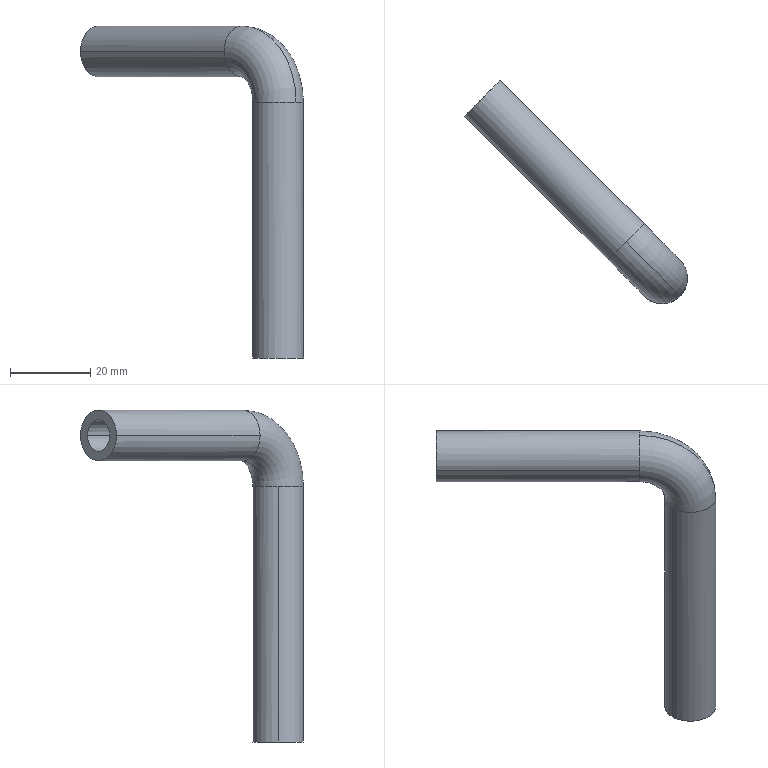Part | STEP file | Tube-500X095_1^Tube_6-P01_ASSEMBLY_KOMBAJN_OWOCOWY-003V11_Tube .500in OD X .095in Wall | 1 solid | 14 faces | box 55.673 x 55.673 x 82.885 mm | volume 10488 mm3 | cylinder 8 | torus 4 | plane 2 | commonest cylinder face diameters 7.874 x4 12.7 x4
STEP:
#1=CARTESIAN_POINT('',(0.,0.,0.));
#2=DIRECTION('',(0.,0.,1.));
#3=DIRECTION('',(1.,0.,0.));
#4=AXIS2_PLACEMENT_3D('',#1,#2,#3);
#5=CARTESIAN_POINT('',(3.937,0.,63.835));
#6=VERTEX_POINT('',#5);
#7=CARTESIAN_POINT('',(-2.784,2.784,63.835));
#8=VERTEX_POINT('',#7);
#9=CARTESIAN_POINT('',(0.,0.,63.835));
#10=DIRECTION('',(0.,0.,1.));
#11=DIRECTION('',(-1.,0.,0.));
#12=AXIS2_PLACEMENT_3D('',#9,#10,#11);
#13=CIRCLE('',#12,3.937);
#14=CARTESIAN_POINT('',(-8.98,8.98,63.835));
#15=DIRECTION('',(-0.7071,-0.7071,0.));
#16=DIRECTION('',(0.7071,-0.7071,0.));
#17=AXIS2_PLACEMENT_3D('',#14,#15,#16);
#18=TOROIDAL_SURFACE('',#17,12.7,3.937);
#19=CARTESIAN_POINT('',(0.,8.639));
#20=DIRECTION('',(0.,-1.));
#21=VECTOR('',#20,1.);
#22=LINE('',#19,#21);
#23=(GEOMETRIC_REPRESENTATION_CONTEXT(2)PARAMETRIC_REPRESENTATION_CONTEXT()REPRESENTATION_CONTEXT('',''));
#24=DEFINITIONAL_REPRESENTATION('',(#22),#23);
#25=PCURVE('',#18,#24);
#26=CARTESIAN_POINT('',(0.,0.,63.835));
#27=DIRECTION('',(0.,0.,-1.));
#28=DIRECTION('',(-1.,0.,0.));
#29=AXIS2_PLACEMENT_3D('',#26,#27,#28);
#30=CYLINDRICAL_SURFACE('',#29,3.937);
#31=CARTESIAN_POINT('',(6.283,0.));
#32=DIRECTION('',(-1.,0.));
#33=VECTOR('',#32,1.);
#34=LINE('',#31,#33);
#35=(GEOMETRIC_REPRESENTATION_CONTEXT(2)PARAMETRIC_REPRESENTATION_CONTEXT()REPRESENTATION_CONTEXT('',''));
#36=DEFINITIONAL_REPRESENTATION('',(#34),#35);
#37=PCURVE('',#30,#36);
#38=SURFACE_CURVE('',#13,(#25,#37),.PCURVE_S1.);
#39=EDGE_CURVE('',#6,#8,#38,.T.);
#40=ORIENTED_EDGE('',*,*,#39,.T.);
#41=CARTESIAN_POINT('',(-8.98,8.98,72.598));
#42=VERTEX_POINT('',#41);
#43=CARTESIAN_POINT('',(-8.98,8.98,63.835));
#44=DIRECTION('',(-0.7071,-0.7071,0.));
#45=DIRECTION('',(0.7071,-0.7071,0.));
#46=AXIS2_PLACEMENT_3D('',#43,#44,#45);
#47=CIRCLE('',#46,8.763);
#48=CARTESIAN_POINT('',(0.,3.142));
#49=DIRECTION('',(1.,0.));
#50=VECTOR('',#49,1.);
#51=LINE('',#48,#50);
#52=(GEOMETRIC_REPRESENTATION_CONTEXT(2)PARAMETRIC_REPRESENTATION_CONTEXT()REPRESENTATION_CONTEXT('',''));
#53=DEFINITIONAL_REPRESENTATION('',(#51),#52);
#54=PCURVE('',#18,#53);
#55=CARTESIAN_POINT('',(-8.98,8.98,63.835));
#56=DIRECTION('',(-0.7071,-0.7071,0.));
#57=DIRECTION('',(0.7071,-0.7071,0.));
#58=AXIS2_PLACEMENT_3D('',#55,#56,#57);
#59=TOROIDAL_SURFACE('',#58,12.7,3.937);
#60=CARTESIAN_POINT('',(0.,3.142));
#61=DIRECTION('',(1.,0.));
#62=VECTOR('',#61,1.);
#63=LINE('',#60,#62);
#64=(GEOMETRIC_REPRESENTATION_CONTEXT(2)PARAMETRIC_REPRESENTATION_CONTEXT()REPRESENTATION_CONTEXT('',''));
#65=DEFINITIONAL_REPRESENTATION('',(#63),#64);
#66=PCURVE('',#59,#65);
#67=SURFACE_CURVE('',#47,(#54,#66),.PCURVE_S1.);
#68=EDGE_CURVE('',#8,#42,#67,.T.);
#69=ORIENTED_EDGE('',*,*,#68,.T.);
#70=CARTESIAN_POINT('',(-6.196,11.764,76.535));
#71=VERTEX_POINT('',#70);
#72=CARTESIAN_POINT('',(-8.98,8.98,76.535));
#73=DIRECTION('',(-0.7071,0.7071,0.));
#74=DIRECTION('',(-0.7071,-0.7071,0.));
#75=AXIS2_PLACEMENT_3D('',#72,#73,#74);
#76=CIRCLE('',#75,3.937);
#77=CARTESIAN_POINT('',(1.571,7.854));
#78=DIRECTION('',(0.,-1.));
#79=VECTOR('',#78,1.);
#80=LINE('',#77,#79);
#81=(GEOMETRIC_REPRESENTATION_CONTEXT(2)PARAMETRIC_REPRESENTATION_CONTEXT()REPRESENTATION_CONTEXT('',''));
#82=DEFINITIONAL_REPRESENTATION('',(#80),#81);
#83=PCURVE('',#18,#82);
#84=CARTESIAN_POINT('',(-8.98,8.98,76.535));
#85=DIRECTION('',(-0.7071,0.7071,0.));
#86=DIRECTION('',(-0.7071,-0.7071,0.));
#87=AXIS2_PLACEMENT_3D('',#84,#85,#86);
#88=CYLINDRICAL_SURFACE('',#87,3.937);
#89=CARTESIAN_POINT('',(0.,0.));
#90=DIRECTION('',(1.,0.));
#91=VECTOR('',#90,1.);
#92=LINE('',#89,#91);
#93=(GEOMETRIC_REPRESENTATION_CONTEXT(2)PARAMETRIC_REPRESENTATION_CONTEXT()REPRESENTATION_CONTEXT('',''));
#94=DEFINITIONAL_REPRESENTATION('',(#92),#93);
#95=PCURVE('',#88,#94);
#96=SURFACE_CURVE('',#76,(#83,#95),.PCURVE_S1.);
#97=EDGE_CURVE('',#71,#42,#96,.T.);
#98=ORIENTED_EDGE('',*,*,#97,.F.);
#99=CARTESIAN_POINT('',(-8.98,8.98,80.472));
#100=VERTEX_POINT('',#99);
#101=CARTESIAN_POINT('',(-8.98,8.98,76.535));
#102=DIRECTION('',(-0.7071,0.7071,0.));
#103=DIRECTION('',(-0.7071,-0.7071,0.));
#104=AXIS2_PLACEMENT_3D('',#101,#102,#103);
#105=CIRCLE('',#104,3.937);
#106=CARTESIAN_POINT('',(1.571,7.854));
#107=DIRECTION('',(0.,-1.));
#108=VECTOR('',#107,1.);
#109=LINE('',#106,#108);
#110=(GEOMETRIC_REPRESENTATION_CONTEXT(2)PARAMETRIC_REPRESENTATION_CONTEXT()REPRESENTATION_CONTEXT('',''));
#111=DEFINITIONAL_REPRESENTATION('',(#109),#110);
#112=PCURVE('',#18,#111);
#113=CARTESIAN_POINT('',(-8.98,8.98,76.535));
#114=DIRECTION('',(-0.7071,0.7071,0.));
#115=DIRECTION('',(-0.7071,-0.7071,0.));
#116=AXIS2_PLACEMENT_3D('',#113,#114,#115);
#117=CYLINDRICAL_SURFACE('',#116,3.937);
#118=CARTESIAN_POINT('',(0.,0.));
#119=DIRECTION('',(1.,0.));
#120=VECTOR('',#119,1.);
#121=LINE('',#118,#120);
#122=(GEOMETRIC_REPRESENTATION_CONTEXT(2)PARAMETRIC_REPRESENTATION_CONTEXT()REPRESENTATION_CONTEXT('',''));
#123=DEFINITIONAL_REPRESENTATION('',(#121),#122);
#124=PCURVE('',#117,#123);
#125=SURFACE_CURVE('',#105,(#112,#124),.PCURVE_S1.);
#126=EDGE_CURVE('',#100,#71,#125,.T.);
#127=ORIENTED_EDGE('',*,*,#126,.F.);
#128=CARTESIAN_POINT('',(2.784,-2.784,63.835));
#129=VERTEX_POINT('',#128);
#130=CARTESIAN_POINT('',(-8.98,8.98,63.835));
#131=DIRECTION('',(-0.7071,-0.7071,0.));
#132=DIRECTION('',(0.7071,-0.7071,0.));
#133=AXIS2_PLACEMENT_3D('',#130,#131,#132);
#134=CIRCLE('',#133,16.637);
#135=CARTESIAN_POINT('',(0.,6.283));
#136=DIRECTION('',(1.,0.));
#137=VECTOR('',#136,1.);
#138=LINE('',#135,#137);
#139=(GEOMETRIC_REPRESENTATION_CONTEXT(2)PARAMETRIC_REPRESENTATION_CONTEXT()REPRESENTATION_CONTEXT('',''));
#140=DEFINITIONAL_REPRESENTATION('',(#138),#139);
#141=PCURVE('',#18,#140);
#142=CARTESIAN_POINT('',(0.,0.));
#143=DIRECTION('',(1.,0.));
#144=VECTOR('',#143,1.);
#145=LINE('',#142,#144);
#146=(GEOMETRIC_REPRESENTATION_CONTEXT(2)PARAMETRIC_REPRESENTATION_CONTEXT()REPRESENTATION_CONTEXT('',''));
#147=DEFINITIONAL_REPRESENTATION('',(#145),#146);
#148=PCURVE('',#59,#147);
#149=SURFACE_CURVE('',#134,(#141,#148),.PCURVE_S1.);
#150=EDGE_CURVE('',#129,#100,#149,.T.);
#151=ORIENTED_EDGE('',*,*,#150,.F.);
#152=CARTESIAN_POINT('',(0.,0.,63.835));
#153=DIRECTION('',(0.,0.,1.));
#154=DIRECTION('',(-1.,0.,0.));
#155=AXIS2_PLACEMENT_3D('',#152,#153,#154);
#156=CIRCLE('',#155,3.937);
#157=CARTESIAN_POINT('',(0.,8.639));
#158=DIRECTION('',(0.,-1.));
#159=VECTOR('',#158,1.);
#160=LINE('',#157,#159);
#161=(GEOMETRIC_REPRESENTATION_CONTEXT(2)PARAMETRIC_REPRESENTATION_CONTEXT()REPRESENTATION_CONTEXT('',''));
#162=DEFINITIONAL_REPRESENTATION('',(#160),#161);
#163=PCURVE('',#18,#162);
#164=CARTESIAN_POINT('',(0.,0.,63.835));
#165=DIRECTION('',(0.,0.,-1.));
#166=DIRECTION('',(-1.,0.,0.));
#167=AXIS2_PLACEMENT_3D('',#164,#165,#166);
#168=CYLINDRICAL_SURFACE('',#167,3.937);
#169=CARTESIAN_POINT('',(6.283,0.));
#170=DIRECTION('',(-1.,0.));
#171=VECTOR('',#170,1.);
#172=LINE('',#169,#171);
#173=(GEOMETRIC_REPRESENTATION_CONTEXT(2)PARAMETRIC_REPRESENTATION_CONTEXT()REPRESENTATION_CONTEXT('',''));
#174=DEFINITIONAL_REPRESENTATION('',(#172),#173);
#175=PCURVE('',#168,#174);
#176=SURFACE_CURVE('',#156,(#163,#175),.PCURVE_S1.);
#177=EDGE_CURVE('',#129,#6,#176,.T.);
#178=ORIENTED_EDGE('',*,*,#177,.T.);
#179=EDGE_LOOP('',(#40,#69,#98,#127,#151,#178));
#180=FACE_BOUND('',#179,.F.);
#181=ADVANCED_FACE('',(#180),#18,.F.);
#182=CARTESIAN_POINT('',(-6.35,0.,63.835));
#183=VERTEX_POINT('',#182);
#184=CARTESIAN_POINT('',(4.49,-4.49,63.835));
#185=VERTEX_POINT('',#184);
#186=CARTESIAN_POINT('',(0.,0.,63.835));
#187=DIRECTION('',(0.,0.,1.));
#188=DIRECTION('',(1.,0.,0.));
#189=AXIS2_PLACEMENT_3D('',#186,#187,#188);
#190=CIRCLE('',#189,6.35);
#191=CARTESIAN_POINT('',(-8.98,8.98,63.835));
#192=DIRECTION('',(-0.7071,-0.7071,0.));
#193=DIRECTION('',(0.7071,-0.7071,0.));
#194=AXIS2_PLACEMENT_3D('',#191,#192,#193);
#195=TOROIDAL_SURFACE('',#194,12.7,6.35);
#196=CARTESIAN_POINT('',(0.,5.498));
#197=DIRECTION('',(0.,-1.));
#198=VECTOR('',#197,1.);
#199=LINE('',#196,#198);
#200=(GEOMETRIC_REPRESENTATION_CONTEXT(2)PARAMETRIC_REPRESENTATION_CONTEXT()REPRESENTATION_CONTEXT('',''));
#201=DEFINITIONAL_REPRESENTATION('',(#199),#200);
#202=PCURVE('',#195,#201);
#203=CARTESIAN_POINT('',(0.,0.,63.835));
#204=DIRECTION('',(0.,0.,-1.));
#205=DIRECTION('',(-1.,0.,0.));
#206=AXIS2_PLACEMENT_3D('',#203,#204,#205);
#207=CYLINDRICAL_SURFACE('',#206,6.35);
#208=CARTESIAN_POINT('',(9.425,0.));
#209=DIRECTION('',(-1.,0.));
#210=VECTOR('',#209,1.);
#211=LINE('',#208,#210);
#212=(GEOMETRIC_REPRESENTATION_CONTEXT(2)PARAMETRIC_REPRESENTATION_CONTEXT()REPRESENTATION_CONTEXT('',''));
#213=DEFINITIONAL_REPRESENTATION('',(#211),#212);
#214=PCURVE('',#207,#213);
#215=SURFACE_CURVE('',#190,(#202,#214),.PCURVE_S1.);
#216=EDGE_CURVE('',#183,#185,#215,.T.);
#217=ORIENTED_EDGE('',*,*,#216,.T.);
#218=CARTESIAN_POINT('',(-8.98,8.98,82.885));
#219=VERTEX_POINT('',#218);
#220=CARTESIAN_POINT('',(-8.98,8.98,63.835));
#221=DIRECTION('',(-0.7071,-0.7071,0.));
#222=DIRECTION('',(0.7071,-0.7071,0.));
#223=AXIS2_PLACEMENT_3D('',#220,#221,#222);
#224=CIRCLE('',#223,19.05);
#225=CARTESIAN_POINT('',(0.,0.));
#226=DIRECTION('',(1.,0.));
#227=VECTOR('',#226,1.);
#228=LINE('',#225,#227);
#229=(GEOMETRIC_REPRESENTATION_CONTEXT(2)PARAMETRIC_REPRESENTATION_CONTEXT()REPRESENTATION_CONTEXT('',''));
#230=DEFINITIONAL_REPRESENTATION('',(#228),#229);
#231=PCURVE('',#195,#230);
#232=CARTESIAN_POINT('',(-8.98,8.98,63.835));
#233=DIRECTION('',(-0.7071,-0.7071,0.));
#234=DIRECTION('',(0.7071,-0.7071,0.));
#235=AXIS2_PLACEMENT_3D('',#232,#233,#234);
#236=TOROIDAL_SURFACE('',#235,12.7,6.35);
#237=CARTESIAN_POINT('',(0.,6.283));
#238=CARTESIAN_POINT('',(0.0238,6.283));
#239=CARTESIAN_POINT('',(0.0714,6.283));
#240=CARTESIAN_POINT('',(0.1428,6.283));
#241=CARTESIAN_POINT('',(0.2142,6.283));
#242=CARTESIAN_POINT('',(0.2856,6.283));
#243=CARTESIAN_POINT('',(0.357,6.283));
#244=CARTESIAN_POINT('',(0.4284,6.283));
#245=CARTESIAN_POINT('',(0.4998,6.283));
#246=CARTESIAN_POINT('',(0.5712,6.283));
#247=CARTESIAN_POINT('',(0.6426,6.283));
#248=CARTESIAN_POINT('',(0.714,6.283));
#249=CARTESIAN_POINT('',(0.7854,6.283));
#250=CARTESIAN_POINT('',(0.8568,6.283));
#251=CARTESIAN_POINT('',(0.9282,6.283));
#252=CARTESIAN_POINT('',(0.9996,6.283));
#253=CARTESIAN_POINT('',(1.071,6.283));
#254=CARTESIAN_POINT('',(1.142,6.283));
#255=CARTESIAN_POINT('',(1.214,6.283));
#256=CARTESIAN_POINT('',(1.285,6.283));
#257=CARTESIAN_POINT('',(1.357,6.283));
#258=CARTESIAN_POINT('',(1.428,6.283));
#259=CARTESIAN_POINT('',(1.499,6.283));
#260=CARTESIAN_POINT('',(1.547,6.283));
#261=CARTESIAN_POINT('',(1.571,6.283));
#262=B_SPLINE_CURVE_WITH_KNOTS('',3,(#237,#238,#239,#240,#241,#242,#243,#244,#245,#246,#247,#248,#249,#250,#251,#252,#253,#254,#255,#256,#257,#258,#259,#260,#261),.UNSPECIFIED.,.F.,.F.,(4,1,1,1,1,1,1,1,1,1,1,1,1,1,1,1,1,1,1,1,1,1,4),(0.,0.0714,0.1428,0.2142,0.2856,0.357,0.4284,0.4998,0.5712,0.6426,0.714,0.7854,0.8568,0.9282,0.9996,1.071,1.142,1.214,1.285,1.357,1.428,1.499,1.571),.QUASI_UNIFORM_KNOTS.);
#263=(GEOMETRIC_REPRESENTATION_CONTEXT(2)PARAMETRIC_REPRESENTATION_CONTEXT()REPRESENTATION_CONTEXT('',''));
#264=DEFINITIONAL_REPRESENTATION('',(#262),#263);
#265=PCURVE('',#236,#264);
#266=SURFACE_CURVE('',#224,(#231,#265),.PCURVE_S1.);
#267=EDGE_CURVE('',#185,#219,#266,.T.);
#268=ORIENTED_EDGE('',*,*,#267,.T.);
#269=CARTESIAN_POINT('',(-13.47,4.49,76.535));
#270=VERTEX_POINT('',#269);
#271=CARTESIAN_POINT('',(-8.98,8.98,76.535));
#272=DIRECTION('',(-0.7071,0.7071,0.));
#273=DIRECTION('',(0.5,0.5,0.7071));
#274=AXIS2_PLACEMENT_3D('',#271,#272,#273);
#275=CIRCLE('',#274,6.35);
#276=CARTESIAN_POINT('',(1.571,5.498));
#277=DIRECTION('',(0.,-1.));
#278=VECTOR('',#277,1.);
#279=LINE('',#276,#278);
#280=(GEOMETRIC_REPRESENTATION_CONTEXT(2)PARAMETRIC_REPRESENTATION_CONTEXT()REPRESENTATION_CONTEXT('',''));
#281=DEFINITIONAL_REPRESENTATION('',(#279),#280);
#282=PCURVE('',#195,#281);
#283=CARTESIAN_POINT('',(-8.98,8.98,76.535));
#284=DIRECTION('',(-0.7071,0.7071,0.));
#285=DIRECTION('',(-0.7071,-0.7071,0.));
#286=AXIS2_PLACEMENT_3D('',#283,#284,#285);
#287=CYLINDRICAL_SURFACE('',#286,6.35);
#288=CARTESIAN_POINT('',(-3.927,0.));
#289=DIRECTION('',(1.,0.));
#290=VECTOR('',#289,1.);
#291=LINE('',#288,#290);
#292=(GEOMETRIC_REPRESENTATION_CONTEXT(2)PARAMETRIC_REPRESENTATION_CONTEXT()REPRESENTATION_CONTEXT('',''));
#293=DEFINITIONAL_REPRESENTATION('',(#291),#292);
#294=PCURVE('',#287,#293);
#295=SURFACE_CURVE('',#275,(#282,#294),.PCURVE_S1.);
#296=EDGE_CURVE('',#270,#219,#295,.T.);
#297=ORIENTED_EDGE('',*,*,#296,.F.);
#298=CARTESIAN_POINT('',(-8.98,8.98,70.185));
#299=VERTEX_POINT('',#298);
#300=CARTESIAN_POINT('',(-8.98,8.98,76.535));
#301=DIRECTION('',(-0.7071,0.7071,0.));
#302=DIRECTION('',(0.5,0.5,0.7071));
#303=AXIS2_PLACEMENT_3D('',#300,#301,#302);
#304=CIRCLE('',#303,6.35);
#305=CARTESIAN_POINT('',(1.571,5.498));
#306=DIRECTION('',(0.,-1.));
#307=VECTOR('',#306,1.);
#308=LINE('',#305,#307);
#309=(GEOMETRIC_REPRESENTATION_CONTEXT(2)PARAMETRIC_REPRESENTATION_CONTEXT()REPRESENTATION_CONTEXT('',''));
#310=DEFINITIONAL_REPRESENTATION('',(#308),#309);
#311=PCURVE('',#195,#310);
#312=CARTESIAN_POINT('',(-8.98,8.98,76.535));
#313=DIRECTION('',(-0.7071,0.7071,0.));
#314=DIRECTION('',(-0.7071,-0.7071,0.));
#315=AXIS2_PLACEMENT_3D('',#312,#313,#314);
#316=CYLINDRICAL_SURFACE('',#315,6.35);
#317=CARTESIAN_POINT('',(2.356,0.));
#318=DIRECTION('',(1.,0.));
#319=VECTOR('',#318,1.);
#320=LINE('',#317,#319);
#321=(GEOMETRIC_REPRESENTATION_CONTEXT(2)PARAMETRIC_REPRESENTATION_CONTEXT()REPRESENTATION_CONTEXT('',''));
#322=DEFINITIONAL_REPRESENTATION('',(#320),#321);
#323=PCURVE('',#316,#322);
#324=SURFACE_CURVE('',#304,(#311,#323),.PCURVE_S1.);
#325=EDGE_CURVE('',#299,#270,#324,.T.);
#326=ORIENTED_EDGE('',*,*,#325,.F.);
#327=CARTESIAN_POINT('',(-4.49,4.49,63.835));
#328=VERTEX_POINT('',#327);
#329=CARTESIAN_POINT('',(-8.98,8.98,63.835));
#330=DIRECTION('',(-0.7071,-0.7071,0.));
#331=DIRECTION('',(0.7071,-0.7071,0.));
#332=AXIS2_PLACEMENT_3D('',#329,#330,#331);
#333=CIRCLE('',#332,6.35);
#334=CARTESIAN_POINT('',(0.,3.142));
#335=DIRECTION('',(1.,0.));
#336=VECTOR('',#335,1.);
#337=LINE('',#334,#336);
#338=(GEOMETRIC_REPRESENTATION_CONTEXT(2)PARAMETRIC_REPRESENTATION_CONTEXT()REPRESENTATION_CONTEXT('',''));
#339=DEFINITIONAL_REPRESENTATION('',(#337),#338);
#340=PCURVE('',#195,#339);
#341=CARTESIAN_POINT('',(0.,3.142));
#342=DIRECTION('',(1.,0.));
#343=VECTOR('',#342,1.);
#344=LINE('',#341,#343);
#345=(GEOMETRIC_REPRESENTATION_CONTEXT(2)PARAMETRIC_REPRESENTATION_CONTEXT()REPRESENTATION_CONTEXT('',''));
#346=DEFINITIONAL_REPRESENTATION('',(#344),#345);
#347=PCURVE('',#236,#346);
#348=SURFACE_CURVE('',#333,(#340,#347),.PCURVE_S1.);
#349=EDGE_CURVE('',#328,#299,#348,.T.);
#350=ORIENTED_EDGE('',*,*,#349,.F.);
#351=CARTESIAN_POINT('',(0.,0.,63.835));
#352=DIRECTION('',(0.,0.,1.));
#353=DIRECTION('',(1.,0.,0.));
#354=AXIS2_PLACEMENT_3D('',#351,#352,#353);
#355=CIRCLE('',#354,6.35);
#356=CARTESIAN_POINT('',(0.,5.498));
#357=DIRECTION('',(0.,-1.));
#358=VECTOR('',#357,1.);
#359=LINE('',#356,#358);
#360=(GEOMETRIC_REPRESENTATION_CONTEXT(2)PARAMETRIC_REPRESENTATION_CONTEXT()REPRESENTATION_CONTEXT('',''));
#361=DEFINITIONAL_REPRESENTATION('',(#359),#360);
#362=PCURVE('',#195,#361);
#363=CARTESIAN_POINT('',(0.,0.,63.835));
#364=DIRECTION('',(0.,0.,-1.));
#365=DIRECTION('',(-1.,0.,0.));
#366=AXIS2_PLACEMENT_3D('',#363,#364,#365);
#367=CYLINDRICAL_SURFACE('',#366,6.35);
#368=CARTESIAN_POINT('',(3.142,0.));
#369=DIRECTION('',(-1.,0.));
#370=VECTOR('',#369,1.);
#371=LINE('',#368,#370);
#372=(GEOMETRIC_REPRESENTATION_CONTEXT(2)PARAMETRIC_REPRESENTATION_CONTEXT()REPRESENTATION_CONTEXT('',''));
#373=DEFINITIONAL_REPRESENTATION('',(#371),#372);
#374=PCURVE('',#367,#373);
#375=SURFACE_CURVE('',#355,(#362,#374),.PCURVE_S1.);
#376=EDGE_CURVE('',#328,#183,#375,.T.);
#377=ORIENTED_EDGE('',*,*,#376,.T.);
#378=EDGE_LOOP('',(#217,#268,#297,#326,#350,#377));
#379=FACE_BOUND('',#378,.T.);
#380=ADVANCED_FACE('',(#379),#195,.T.);
#381=CARTESIAN_POINT('',(-3.937,0.,63.835));
#382=VERTEX_POINT('',#381);
#383=CARTESIAN_POINT('',(-3.937,0.,0.));
#384=VERTEX_POINT('',#383);
#385=CARTESIAN_POINT('',(-3.937,0.,63.835));
#386=DIRECTION('',(0.,0.,-1.));
#387=VECTOR('',#386,1.);
#388=LINE('',#385,#387);
#389=CARTESIAN_POINT('',(6.283,0.));
#390=DIRECTION('',(0.,1.));
#391=VECTOR('',#390,1.);
#392=LINE('',#389,#391);
#393=(GEOMETRIC_REPRESENTATION_CONTEXT(2)PARAMETRIC_REPRESENTATION_CONTEXT()REPRESENTATION_CONTEXT('',''));
#394=DEFINITIONAL_REPRESENTATION('',(#392),#393);
#395=PCURVE('',#168,#394);
#396=CARTESIAN_POINT('',(0.,0.));
#397=DIRECTION('',(0.,1.));
#398=VECTOR('',#397,1.);
#399=LINE('',#396,#398);
#400=(GEOMETRIC_REPRESENTATION_CONTEXT(2)PARAMETRIC_REPRESENTATION_CONTEXT()REPRESENTATION_CONTEXT('',''));
#401=DEFINITIONAL_REPRESENTATION('',(#399),#400);
#402=PCURVE('',#30,#401);
#403=SURFACE_CURVE('',#388,(#395,#402),.PCURVE_S1.);
#404=EDGE_CURVE('',#382,#384,#403,.T.);
#405=ORIENTED_EDGE('',*,*,#404,.T.);
#406=CARTESIAN_POINT('',(3.937,0.,0.));
#407=VERTEX_POINT('',#406);
#408=CARTESIAN_POINT('',(0.,0.,0.));
#409=DIRECTION('',(0.,0.,1.));
#410=DIRECTION('',(1.,0.,0.));
#411=AXIS2_PLACEMENT_3D('',#408,#409,#410);
#412=CIRCLE('',#411,3.937);
#413=CARTESIAN_POINT('',(9.425,63.835));
#414=DIRECTION('',(-1.,0.));
#415=VECTOR('',#414,1.);
#416=LINE('',#413,#415);
#417=(GEOMETRIC_REPRESENTATION_CONTEXT(2)PARAMETRIC_REPRESENTATION_CONTEXT()REPRESENTATION_CONTEXT('',''));
#418=DEFINITIONAL_REPRESENTATION('',(#416),#417);
#419=PCURVE('',#168,#418);
#420=CARTESIAN_POINT('',(0.,0.,0.));
#421=DIRECTION('',(0.,0.,1.));
#422=DIRECTION('',(1.,0.,0.));
#423=AXIS2_PLACEMENT_3D('',#420,#421,#422);
#424=PLANE('',#423);
#425=CARTESIAN_POINT('',(0.,0.));
#426=DIRECTION('',(1.,0.));
#427=AXIS2_PLACEMENT_2D('',#425,#426);
#428=CIRCLE('',#427,3.937);
#429=(GEOMETRIC_REPRESENTATION_CONTEXT(2)PARAMETRIC_REPRESENTATION_CONTEXT()REPRESENTATION_CONTEXT('',''));
#430=DEFINITIONAL_REPRESENTATION('',(#428),#429);
#431=PCURVE('',#424,#430);
#432=SURFACE_CURVE('',#412,(#419,#431),.PCURVE_S1.);
#433=EDGE_CURVE('',#384,#407,#432,.T.);
#434=ORIENTED_EDGE('',*,*,#433,.T.);
#435=CARTESIAN_POINT('',(3.937,0.,63.835));
#436=DIRECTION('',(0.,0.,-1.));
#437=VECTOR('',#436,1.);
#438=LINE('',#435,#437);
#439=CARTESIAN_POINT('',(3.142,0.));
#440=DIRECTION('',(0.,1.));
#441=VECTOR('',#440,1.);
#442=LINE('',#439,#441);
#443=(GEOMETRIC_REPRESENTATION_CONTEXT(2)PARAMETRIC_REPRESENTATION_CONTEXT()REPRESENTATION_CONTEXT('',''));
#444=DEFINITIONAL_REPRESENTATION('',(#442),#443);
#445=PCURVE('',#168,#444);
#446=CARTESIAN_POINT('',(3.142,0.));
#447=DIRECTION('',(0.,1.));
#448=VECTOR('',#447,1.);
#449=LINE('',#446,#448);
#450=(GEOMETRIC_REPRESENTATION_CONTEXT(2)PARAMETRIC_REPRESENTATION_CONTEXT()REPRESENTATION_CONTEXT('',''));
#451=DEFINITIONAL_REPRESENTATION('',(#449),#450);
#452=PCURVE('',#30,#451);
#453=SURFACE_CURVE('',#438,(#445,#452),.PCURVE_S1.);
#454=EDGE_CURVE('',#6,#407,#453,.T.);
#455=ORIENTED_EDGE('',*,*,#454,.F.);
#456=ORIENTED_EDGE('',*,*,#177,.F.);
#457=CARTESIAN_POINT('',(0.,0.,63.835));
#458=DIRECTION('',(0.,0.,1.));
#459=DIRECTION('',(-1.,0.,0.));
#460=AXIS2_PLACEMENT_3D('',#457,#458,#459);
#461=CIRCLE('',#460,3.937);
#462=CARTESIAN_POINT('',(6.283,0.));
#463=DIRECTION('',(-1.,0.));
#464=VECTOR('',#463,1.);
#465=LINE('',#462,#464);
#466=(GEOMETRIC_REPRESENTATION_CONTEXT(2)PARAMETRIC_REPRESENTATION_CONTEXT()REPRESENTATION_CONTEXT('',''));
#467=DEFINITIONAL_REPRESENTATION('',(#465),#466);
#468=PCURVE('',#168,#467);
#469=CARTESIAN_POINT('',(0.,2.356));
#470=DIRECTION('',(0.,-1.));
#471=VECTOR('',#470,1.);
#472=LINE('',#469,#471);
#473=(GEOMETRIC_REPRESENTATION_CONTEXT(2)PARAMETRIC_REPRESENTATION_CONTEXT()REPRESENTATION_CONTEXT('',''));
#474=DEFINITIONAL_REPRESENTATION('',(#472),#473);
#475=PCURVE('',#59,#474);
#476=SURFACE_CURVE('',#461,(#468,#475),.PCURVE_S1.);
#477=EDGE_CURVE('',#382,#129,#476,.T.);
#478=ORIENTED_EDGE('',*,*,#477,.F.);
#479=EDGE_LOOP('',(#405,#434,#455,#456,#478));
#480=FACE_BOUND('',#479,.F.);
#481=ADVANCED_FACE('',(#480),#168,.F.);
#482=CARTESIAN_POINT('',(-11.764,6.196,76.535));
#483=VERTEX_POINT('',#482);
#484=CARTESIAN_POINT('',(-8.98,8.98,76.535));
#485=DIRECTION('',(-0.7071,0.7071,0.));
#486=DIRECTION('',(-0.7071,-0.7071,0.));
#487=AXIS2_PLACEMENT_3D('',#484,#485,#486);
#488=CIRCLE('',#487,3.937);
#489=CARTESIAN_POINT('',(0.,0.));
#490=DIRECTION('',(1.,0.));
#491=VECTOR('',#490,1.);
#492=LINE('',#489,#491);
#493=(GEOMETRIC_REPRESENTATION_CONTEXT(2)PARAMETRIC_REPRESENTATION_CONTEXT()REPRESENTATION_CONTEXT('',''));
#494=DEFINITIONAL_REPRESENTATION('',(#492),#493);
#495=PCURVE('',#88,#494);
#496=CARTESIAN_POINT('',(1.571,7.854));
#497=DIRECTION('',(0.,-1.));
#498=VECTOR('',#497,1.);
#499=LINE('',#496,#498);
#500=(GEOMETRIC_REPRESENTATION_CONTEXT(2)PARAMETRIC_REPRESENTATION_CONTEXT()REPRESENTATION_CONTEXT('',''));
#501=DEFINITIONAL_REPRESENTATION('',(#499),#500);
#502=PCURVE('',#59,#501);
#503=SURFACE_CURVE('',#488,(#495,#502),.PCURVE_S1.);
#504=EDGE_CURVE('',#42,#483,#503,.T.);
#505=ORIENTED_EDGE('',*,*,#504,.T.);
#506=CARTESIAN_POINT('',(-47.616,42.049,76.535));
#507=VERTEX_POINT('',#506);
#508=CARTESIAN_POINT('',(-11.764,6.196,76.535));
#509=DIRECTION('',(-0.7071,0.7071,0.));
#510=VECTOR('',#509,1.);
#511=LINE('',#508,#510);
#512=CARTESIAN_POINT('',(6.283,0.));
#513=DIRECTION('',(0.,1.));
#514=VECTOR('',#513,1.);
#515=LINE('',#512,#514);
#516=(GEOMETRIC_REPRESENTATION_CONTEXT(2)PARAMETRIC_REPRESENTATION_CONTEXT()REPRESENTATION_CONTEXT('',''));
#517=DEFINITIONAL_REPRESENTATION('',(#515),#516);
#518=PCURVE('',#88,#517);
#519=CARTESIAN_POINT('',(0.,0.));
#520=DIRECTION('',(0.,1.));
#521=VECTOR('',#520,1.);
#522=LINE('',#519,#521);
#523=(GEOMETRIC_REPRESENTATION_CONTEXT(2)PARAMETRIC_REPRESENTATION_CONTEXT()REPRESENTATION_CONTEXT('',''));
#524=DEFINITIONAL_REPRESENTATION('',(#522),#523);
#525=PCURVE('',#117,#524);
#526=SURFACE_CURVE('',#511,(#518,#525),.PCURVE_S1.);
#527=EDGE_CURVE('',#483,#507,#526,.T.);
#528=ORIENTED_EDGE('',*,*,#527,.T.);
#529=CARTESIAN_POINT('',(-42.049,47.616,76.535));
#530=VERTEX_POINT('',#529);
#531=CARTESIAN_POINT('',(-44.832,44.832,76.535));
#532=DIRECTION('',(-0.7071,0.7071,0.));
#533=DIRECTION('',(-0.7071,-0.7071,0.));
#534=AXIS2_PLACEMENT_3D('',#531,#532,#533);
#535=CIRCLE('',#534,3.937);
#536=CARTESIAN_POINT('',(0.,50.703));
#537=DIRECTION('',(1.,0.));
#538=VECTOR('',#537,1.);
#539=LINE('',#536,#538);
#540=(GEOMETRIC_REPRESENTATION_CONTEXT(2)PARAMETRIC_REPRESENTATION_CONTEXT()REPRESENTATION_CONTEXT('',''));
#541=DEFINITIONAL_REPRESENTATION('',(#539),#540);
#542=PCURVE('',#88,#541);
#543=CARTESIAN_POINT('',(-44.832,44.832,76.535));
#544=DIRECTION('',(-0.7071,0.7071,0.));
#545=DIRECTION('',(0.5,0.5,0.7071));
#546=AXIS2_PLACEMENT_3D('',#543,#544,#545);
#547=PLANE('',#546);
#548=CARTESIAN_POINT('',(0.,0.));
#549=DIRECTION('',(-0.7071,-0.7071));
#550=AXIS2_PLACEMENT_2D('',#548,#549);
#551=CIRCLE('',#550,3.937);
#552=(GEOMETRIC_REPRESENTATION_CONTEXT(2)PARAMETRIC_REPRESENTATION_CONTEXT()REPRESENTATION_CONTEXT('',''));
#553=DEFINITIONAL_REPRESENTATION('',(#551),#552);
#554=PCURVE('',#547,#553);
#555=SURFACE_CURVE('',#535,(#542,#554),.PCURVE_S1.);
#556=EDGE_CURVE('',#530,#507,#555,.T.);
#557=ORIENTED_EDGE('',*,*,#556,.F.);
#558=CARTESIAN_POINT('',(-6.196,11.764,76.535));
#559=DIRECTION('',(-0.7071,0.7071,0.));
#560=VECTOR('',#559,1.);
#561=LINE('',#558,#560);
#562=CARTESIAN_POINT('',(3.142,0.));
#563=DIRECTION('',(0.,1.));
#564=VECTOR('',#563,1.);
#565=LINE('',#562,#564);
#566=(GEOMETRIC_REPRESENTATION_CONTEXT(2)PARAMETRIC_REPRESENTATION_CONTEXT()REPRESENTATION_CONTEXT('',''));
#567=DEFINITIONAL_REPRESENTATION('',(#565),#566);
#568=PCURVE('',#88,#567);
#569=CARTESIAN_POINT('',(3.142,0.));
#570=DIRECTION('',(0.,1.));
#571=VECTOR('',#570,1.);
#572=LINE('',#569,#571);
#573=(GEOMETRIC_REPRESENTATION_CONTEXT(2)PARAMETRIC_REPRESENTATION_CONTEXT()REPRESENTATION_CONTEXT('',''));
#574=DEFINITIONAL_REPRESENTATION('',(#572),#573);
#575=PCURVE('',#117,#574);
#576=SURFACE_CURVE('',#561,(#568,#575),.PCURVE_S1.);
#577=EDGE_CURVE('',#71,#530,#576,.T.);
#578=ORIENTED_EDGE('',*,*,#577,.F.);
#579=ORIENTED_EDGE('',*,*,#97,.T.);
#580=EDGE_LOOP('',(#505,#528,#557,#578,#579));
#581=FACE_BOUND('',#580,.F.);
#582=ADVANCED_FACE('',(#581),#88,.F.);
#583=CARTESIAN_POINT('',(6.35,0.,63.835));
#584=VERTEX_POINT('',#583);
#585=CARTESIAN_POINT('',(0.,0.,63.835));
#586=DIRECTION('',(0.,0.,1.));
#587=DIRECTION('',(1.,0.,0.));
#588=AXIS2_PLACEMENT_3D('',#585,#586,#587);
#589=CIRCLE('',#588,6.35);
#590=CARTESIAN_POINT('',(3.142,0.));
#591=DIRECTION('',(-1.,0.));
#592=VECTOR('',#591,1.);
#593=LINE('',#590,#592);
#594=(GEOMETRIC_REPRESENTATION_CONTEXT(2)PARAMETRIC_REPRESENTATION_CONTEXT()REPRESENTATION_CONTEXT('',''));
#595=DEFINITIONAL_REPRESENTATION('',(#593),#594);
#596=PCURVE('',#367,#595);
#597=CARTESIAN_POINT('',(0.,5.498));
#598=DIRECTION('',(0.,-1.));
#599=VECTOR('',#598,1.);
#600=LINE('',#597,#599);
#601=(GEOMETRIC_REPRESENTATION_CONTEXT(2)PARAMETRIC_REPRESENTATION_CONTEXT()REPRESENTATION_CONTEXT('',''));
#602=DEFINITIONAL_REPRESENTATION('',(#600),#601);
#603=PCURVE('',#236,#602);
#604=SURFACE_CURVE('',#589,(#596,#603),.PCURVE_S1.);
#605=EDGE_CURVE('',#584,#328,#604,.T.);
#606=ORIENTED_EDGE('',*,*,#605,.F.);
#607=CARTESIAN_POINT('',(6.35,0.,0.));
#608=VERTEX_POINT('',#607);
#609=CARTESIAN_POINT('',(6.35,0.,63.835));
#610=DIRECTION('',(0.,0.,-1.));
#611=VECTOR('',#610,1.);
#612=LINE('',#609,#611);
#613=CARTESIAN_POINT('',(3.142,0.));
#614=DIRECTION('',(0.,1.));
#615=VECTOR('',#614,1.);
#616=LINE('',#613,#615);
#617=(GEOMETRIC_REPRESENTATION_CONTEXT(2)PARAMETRIC_REPRESENTATION_CONTEXT()REPRESENTATION_CONTEXT('',''));
#618=DEFINITIONAL_REPRESENTATION('',(#616),#617);
#619=PCURVE('',#367,#618);
#620=CARTESIAN_POINT('',(3.142,0.));
#621=DIRECTION('',(0.,1.));
#622=VECTOR('',#621,1.);
#623=LINE('',#620,#622);
#624=(GEOMETRIC_REPRESENTATION_CONTEXT(2)PARAMETRIC_REPRESENTATION_CONTEXT()REPRESENTATION_CONTEXT('',''));
#625=DEFINITIONAL_REPRESENTATION('',(#623),#624);
#626=PCURVE('',#207,#625);
#627=SURFACE_CURVE('',#612,(#619,#626),.PCURVE_S1.);
#628=EDGE_CURVE('',#584,#608,#627,.T.);
#629=ORIENTED_EDGE('',*,*,#628,.T.);
#630=CARTESIAN_POINT('',(-6.35,0.,0.));
#631=VERTEX_POINT('',#630);
#632=CARTESIAN_POINT('',(0.,0.,0.));
#633=DIRECTION('',(0.,0.,1.));
#634=DIRECTION('',(1.,0.,0.));
#635=AXIS2_PLACEMENT_3D('',#632,#633,#634);
#636=CIRCLE('',#635,6.35);
#637=CARTESIAN_POINT('',(3.142,63.835));
#638=DIRECTION('',(-1.,0.));
#639=VECTOR('',#638,1.);
#640=LINE('',#637,#639);
#641=(GEOMETRIC_REPRESENTATION_CONTEXT(2)PARAMETRIC_REPRESENTATION_CONTEXT()REPRESENTATION_CONTEXT('',''));
#642=DEFINITIONAL_REPRESENTATION('',(#640),#641);
#643=PCURVE('',#367,#642);
#644=CARTESIAN_POINT('',(0.,0.));
#645=DIRECTION('',(1.,0.));
#646=AXIS2_PLACEMENT_2D('',#644,#645);
#647=CIRCLE('',#646,6.35);
#648=(GEOMETRIC_REPRESENTATION_CONTEXT(2)PARAMETRIC_REPRESENTATION_CONTEXT()REPRESENTATION_CONTEXT('',''));
#649=DEFINITIONAL_REPRESENTATION('',(#647),#648);
#650=PCURVE('',#424,#649);
#651=SURFACE_CURVE('',#636,(#643,#650),.PCURVE_S1.);
#652=EDGE_CURVE('',#608,#631,#651,.T.);
#653=ORIENTED_EDGE('',*,*,#652,.T.);
#654=CARTESIAN_POINT('',(-6.35,0.,63.835));
#655=DIRECTION('',(0.,0.,-1.));
#656=VECTOR('',#655,1.);
#657=LINE('',#654,#656);
#658=CARTESIAN_POINT('',(0.,0.));
#659=DIRECTION('',(0.,1.));
#660=VECTOR('',#659,1.);
#661=LINE('',#658,#660);
#662=(GEOMETRIC_REPRESENTATION_CONTEXT(2)PARAMETRIC_REPRESENTATION_CONTEXT()REPRESENTATION_CONTEXT('',''));
#663=DEFINITIONAL_REPRESENTATION('',(#661),#662);
#664=PCURVE('',#367,#663);
#665=CARTESIAN_POINT('',(6.283,0.));
#666=DIRECTION('',(0.,1.));
#667=VECTOR('',#666,1.);
#668=LINE('',#665,#667);
#669=(GEOMETRIC_REPRESENTATION_CONTEXT(2)PARAMETRIC_REPRESENTATION_CONTEXT()REPRESENTATION_CONTEXT('',''));
#670=DEFINITIONAL_REPRESENTATION('',(#668),#669);
#671=PCURVE('',#207,#670);
#672=SURFACE_CURVE('',#657,(#664,#671),.PCURVE_S1.);
#673=EDGE_CURVE('',#183,#631,#672,.T.);
#674=ORIENTED_EDGE('',*,*,#673,.F.);
#675=ORIENTED_EDGE('',*,*,#376,.F.);
#676=EDGE_LOOP('',(#606,#629,#653,#674,#675));
#677=FACE_BOUND('',#676,.T.);
#678=ADVANCED_FACE('',(#677),#367,.T.);
#679=ORIENTED_EDGE('',*,*,#296,.T.);
#680=CARTESIAN_POINT('',(-4.49,13.47,76.535));
#681=VERTEX_POINT('',#680);
#682=CARTESIAN_POINT('',(-8.98,8.98,76.535));
#683=DIRECTION('',(-0.7071,0.7071,0.));
#684=DIRECTION('',(0.5,0.5,0.7071));
#685=AXIS2_PLACEMENT_3D('',#682,#683,#684);
#686=CIRCLE('',#685,6.35);
#687=CARTESIAN_POINT('',(-3.927,0.));
#688=DIRECTION('',(1.,0.));
#689=VECTOR('',#688,1.);
#690=LINE('',#687,#689);
#691=(GEOMETRIC_REPRESENTATION_CONTEXT(2)PARAMETRIC_REPRESENTATION_CONTEXT()REPRESENTATION_CONTEXT('',''));
#692=DEFINITIONAL_REPRESENTATION('',(#690),#691);
#693=PCURVE('',#287,#692);
#694=CARTESIAN_POINT('',(1.571,11.781));
#695=DIRECTION('',(0.,-1.));
#696=VECTOR('',#695,1.);
#697=LINE('',#694,#696);
#698=(GEOMETRIC_REPRESENTATION_CONTEXT(2)PARAMETRIC_REPRESENTATION_CONTEXT()REPRESENTATION_CONTEXT('',''));
#699=DEFINITIONAL_REPRESENTATION('',(#697),#698);
#700=PCURVE('',#236,#699);
#701=SURFACE_CURVE('',#686,(#693,#700),.PCURVE_S1.);
#702=EDGE_CURVE('',#219,#681,#701,.T.);
#703=ORIENTED_EDGE('',*,*,#702,.T.);
#704=CARTESIAN_POINT('',(-40.342,49.323,76.535));
#705=VERTEX_POINT('',#704);
#706=CARTESIAN_POINT('',(-4.49,13.47,76.535));
#707=DIRECTION('',(-0.7071,0.7071,0.));
#708=VECTOR('',#707,1.);
#709=LINE('',#706,#708);
#710=CARTESIAN_POINT('',(3.142,0.));
#711=DIRECTION('',(0.,1.));
#712=VECTOR('',#711,1.);
#713=LINE('',#710,#712);
#714=(GEOMETRIC_REPRESENTATION_CONTEXT(2)PARAMETRIC_REPRESENTATION_CONTEXT()REPRESENTATION_CONTEXT('',''));
#715=DEFINITIONAL_REPRESENTATION('',(#713),#714);
#716=PCURVE('',#287,#715);
#717=CARTESIAN_POINT('',(3.142,0.));
#718=DIRECTION('',(0.,1.));
#719=VECTOR('',#718,1.);
#720=LINE('',#717,#719);
#721=(GEOMETRIC_REPRESENTATION_CONTEXT(2)PARAMETRIC_REPRESENTATION_CONTEXT()REPRESENTATION_CONTEXT('',''));
#722=DEFINITIONAL_REPRESENTATION('',(#720),#721);
#723=PCURVE('',#316,#722);
#724=SURFACE_CURVE('',#709,(#716,#723),.PCURVE_S1.);
#725=EDGE_CURVE('',#681,#705,#724,.T.);
#726=ORIENTED_EDGE('',*,*,#725,.T.);
#727=CARTESIAN_POINT('',(-49.323,40.342,76.535));
#728=VERTEX_POINT('',#727);
#729=CARTESIAN_POINT('',(-44.832,44.832,76.535));
#730=DIRECTION('',(-0.7071,0.7071,0.));
#731=DIRECTION('',(0.5,0.5,0.7071));
#732=AXIS2_PLACEMENT_3D('',#729,#730,#731);
#733=CIRCLE('',#732,6.35);
#734=CARTESIAN_POINT('',(-3.927,50.703));
#735=DIRECTION('',(1.,0.));
#736=VECTOR('',#735,1.);
#737=LINE('',#734,#736);
#738=(GEOMETRIC_REPRESENTATION_CONTEXT(2)PARAMETRIC_REPRESENTATION_CONTEXT()REPRESENTATION_CONTEXT('',''));
#739=DEFINITIONAL_REPRESENTATION('',(#737),#738);
#740=PCURVE('',#287,#739);
#741=CARTESIAN_POINT('',(0.,0.));
#742=DIRECTION('',(1.,0.));
#743=AXIS2_PLACEMENT_2D('',#741,#742);
#744=CIRCLE('',#743,6.35);
#745=(GEOMETRIC_REPRESENTATION_CONTEXT(2)PARAMETRIC_REPRESENTATION_CONTEXT()REPRESENTATION_CONTEXT('',''));
#746=DEFINITIONAL_REPRESENTATION('',(#744),#745);
#747=PCURVE('',#547,#746);
#748=SURFACE_CURVE('',#733,(#740,#747),.PCURVE_S1.);
#749=EDGE_CURVE('',#728,#705,#748,.T.);
#750=ORIENTED_EDGE('',*,*,#749,.F.);
#751=CARTESIAN_POINT('',(-13.47,4.49,76.535));
#752=DIRECTION('',(-0.7071,0.7071,0.));
#753=VECTOR('',#752,1.);
#754=LINE('',#751,#753);
#755=CARTESIAN_POINT('',(0.,0.));
#756=DIRECTION('',(0.,1.));
#757=VECTOR('',#756,1.);
#758=LINE('',#755,#757);
#759=(GEOMETRIC_REPRESENTATION_CONTEXT(2)PARAMETRIC_REPRESENTATION_CONTEXT()REPRESENTATION_CONTEXT('',''));
#760=DEFINITIONAL_REPRESENTATION('',(#758),#759);
#761=PCURVE('',#287,#760);
#762=CARTESIAN_POINT('',(6.283,0.));
#763=DIRECTION('',(0.,1.));
#764=VECTOR('',#763,1.);
#765=LINE('',#762,#764);
#766=(GEOMETRIC_REPRESENTATION_CONTEXT(2)PARAMETRIC_REPRESENTATION_CONTEXT()REPRESENTATION_CONTEXT('',''));
#767=DEFINITIONAL_REPRESENTATION('',(#765),#766);
#768=PCURVE('',#316,#767);
#769=SURFACE_CURVE('',#754,(#761,#768),.PCURVE_S1.);
#770=EDGE_CURVE('',#270,#728,#769,.T.);
#771=ORIENTED_EDGE('',*,*,#770,.F.);
#772=EDGE_LOOP('',(#679,#703,#726,#750,#771));
#773=FACE_BOUND('',#772,.T.);
#774=ADVANCED_FACE('',(#773),#287,.T.);
#775=ORIENTED_EDGE('',*,*,#725,.F.);
#776=CARTESIAN_POINT('',(-8.98,8.98,76.535));
#777=DIRECTION('',(-0.7071,0.7071,0.));
#778=DIRECTION('',(0.5,0.5,0.7071));
#779=AXIS2_PLACEMENT_3D('',#776,#777,#778);
#780=CIRCLE('',#779,6.35);
#781=CARTESIAN_POINT('',(2.356,0.));
#782=DIRECTION('',(1.,0.));
#783=VECTOR('',#782,1.);
#784=LINE('',#781,#783);
#785=(GEOMETRIC_REPRESENTATION_CONTEXT(2)PARAMETRIC_REPRESENTATION_CONTEXT()REPRESENTATION_CONTEXT('',''));
#786=DEFINITIONAL_REPRESENTATION('',(#784),#785);
#787=PCURVE('',#316,#786);
#788=CARTESIAN_POINT('',(1.571,5.498));
#789=DIRECTION('',(0.,-1.));
#790=VECTOR('',#789,1.);
#791=LINE('',#788,#790);
#792=(GEOMETRIC_REPRESENTATION_CONTEXT(2)PARAMETRIC_REPRESENTATION_CONTEXT()REPRESENTATION_CONTEXT('',''));
#793=DEFINITIONAL_REPRESENTATION('',(#791),#792);
#794=PCURVE('',#236,#793);
#795=SURFACE_CURVE('',#780,(#787,#794),.PCURVE_S1.);
#796=EDGE_CURVE('',#681,#299,#795,.T.);
#797=ORIENTED_EDGE('',*,*,#796,.T.);
#798=ORIENTED_EDGE('',*,*,#325,.T.);
#799=ORIENTED_EDGE('',*,*,#770,.T.);
#800=CARTESIAN_POINT('',(-44.832,44.832,76.535));
#801=DIRECTION('',(-0.7071,0.7071,0.));
#802=DIRECTION('',(0.5,0.5,0.7071));
#803=AXIS2_PLACEMENT_3D('',#800,#801,#802);
#804=CIRCLE('',#803,6.35);
#805=CARTESIAN_POINT('',(2.356,50.703));
#806=DIRECTION('',(1.,0.));
#807=VECTOR('',#806,1.);
#808=LINE('',#805,#807);
#809=(GEOMETRIC_REPRESENTATION_CONTEXT(2)PARAMETRIC_REPRESENTATION_CONTEXT()REPRESENTATION_CONTEXT('',''));
#810=DEFINITIONAL_REPRESENTATION('',(#808),#809);
#811=PCURVE('',#316,#810);
#812=CARTESIAN_POINT('',(0.,0.));
#813=DIRECTION('',(1.,0.));
#814=AXIS2_PLACEMENT_2D('',#812,#813);
#815=CIRCLE('',#814,6.35);
#816=(GEOMETRIC_REPRESENTATION_CONTEXT(2)PARAMETRIC_REPRESENTATION_CONTEXT()REPRESENTATION_CONTEXT('',''));
#817=DEFINITIONAL_REPRESENTATION('',(#815),#816);
#818=PCURVE('',#547,#817);
#819=SURFACE_CURVE('',#804,(#811,#818),.PCURVE_S1.);
#820=EDGE_CURVE('',#705,#728,#819,.T.);
#821=ORIENTED_EDGE('',*,*,#820,.F.);
#822=EDGE_LOOP('',(#775,#797,#798,#799,#821));
#823=FACE_BOUND('',#822,.T.);
#824=ADVANCED_FACE('',(#823),#316,.T.);
#825=ORIENTED_EDGE('',*,*,#267,.F.);
#826=CARTESIAN_POINT('',(0.,0.,63.835));
#827=DIRECTION('',(0.,0.,1.));
#828=DIRECTION('',(1.,0.,0.));
#829=AXIS2_PLACEMENT_3D('',#826,#827,#828);
#830=CIRCLE('',#829,6.35);
#831=CARTESIAN_POINT('',(0.,11.781));
#832=DIRECTION('',(0.,-1.));
#833=VECTOR('',#832,1.);
#834=LINE('',#831,#833);
#835=(GEOMETRIC_REPRESENTATION_CONTEXT(2)PARAMETRIC_REPRESENTATION_CONTEXT()REPRESENTATION_CONTEXT('',''));
#836=DEFINITIONAL_REPRESENTATION('',(#834),#835);
#837=PCURVE('',#236,#836);
#838=CARTESIAN_POINT('',(9.425,0.));
#839=DIRECTION('',(-1.,0.));
#840=VECTOR('',#839,1.);
#841=LINE('',#838,#840);
#842=(GEOMETRIC_REPRESENTATION_CONTEXT(2)PARAMETRIC_REPRESENTATION_CONTEXT()REPRESENTATION_CONTEXT('',''));
#843=DEFINITIONAL_REPRESENTATION('',(#841),#842);
#844=PCURVE('',#207,#843);
#845=SURFACE_CURVE('',#830,(#837,#844),.PCURVE_S1.);
#846=EDGE_CURVE('',#185,#584,#845,.T.);
#847=ORIENTED_EDGE('',*,*,#846,.T.);
#848=ORIENTED_EDGE('',*,*,#605,.T.);
#849=ORIENTED_EDGE('',*,*,#349,.T.);
#850=ORIENTED_EDGE('',*,*,#796,.F.);
#851=ORIENTED_EDGE('',*,*,#702,.F.);
#852=EDGE_LOOP('',(#825,#847,#848,#849,#850,#851));
#853=FACE_BOUND('',#852,.T.);
#854=ADVANCED_FACE('',(#853),#236,.T.);
#855=ORIENTED_EDGE('',*,*,#628,.F.);
#856=ORIENTED_EDGE('',*,*,#846,.F.);
#857=ORIENTED_EDGE('',*,*,#216,.F.);
#858=ORIENTED_EDGE('',*,*,#673,.T.);
#859=CARTESIAN_POINT('',(0.,0.,0.));
#860=DIRECTION('',(0.,0.,1.));
#861=DIRECTION('',(1.,0.,0.));
#862=AXIS2_PLACEMENT_3D('',#859,#860,#861);
#863=CIRCLE('',#862,6.35);
#864=CARTESIAN_POINT('',(9.425,63.835));
#865=DIRECTION('',(-1.,0.));
#866=VECTOR('',#865,1.);
#867=LINE('',#864,#866);
#868=(GEOMETRIC_REPRESENTATION_CONTEXT(2)PARAMETRIC_REPRESENTATION_CONTEXT()REPRESENTATION_CONTEXT('',''));
#869=DEFINITIONAL_REPRESENTATION('',(#867),#868);
#870=PCURVE('',#207,#869);
#871=CARTESIAN_POINT('',(0.,0.));
#872=DIRECTION('',(1.,0.));
#873=AXIS2_PLACEMENT_2D('',#871,#872);
#874=CIRCLE('',#873,6.35);
#875=(GEOMETRIC_REPRESENTATION_CONTEXT(2)PARAMETRIC_REPRESENTATION_CONTEXT()REPRESENTATION_CONTEXT('',''));
#876=DEFINITIONAL_REPRESENTATION('',(#874),#875);
#877=PCURVE('',#424,#876);
#878=SURFACE_CURVE('',#863,(#870,#877),.PCURVE_S1.);
#879=EDGE_CURVE('',#631,#608,#878,.T.);
#880=ORIENTED_EDGE('',*,*,#879,.T.);
#881=EDGE_LOOP('',(#855,#856,#857,#858,#880));
#882=FACE_BOUND('',#881,.T.);
#883=ADVANCED_FACE('',(#882),#207,.T.);
#884=CARTESIAN_POINT('',(-44.832,44.832,76.535));
#885=DIRECTION('',(-0.7071,0.7071,0.));
#886=DIRECTION('',(-0.7071,-0.7071,0.));
#887=AXIS2_PLACEMENT_3D('',#884,#885,#886);
#888=CIRCLE('',#887,3.937);
#889=CARTESIAN_POINT('',(0.,0.));
#890=DIRECTION('',(-0.7071,-0.7071));
#891=AXIS2_PLACEMENT_2D('',#889,#890);
#892=CIRCLE('',#891,3.937);
#893=(GEOMETRIC_REPRESENTATION_CONTEXT(2)PARAMETRIC_REPRESENTATION_CONTEXT()REPRESENTATION_CONTEXT('',''));
#894=DEFINITIONAL_REPRESENTATION('',(#892),#893);
#895=PCURVE('',#547,#894);
#896=CARTESIAN_POINT('',(0.,50.703));
#897=DIRECTION('',(1.,0.));
#898=VECTOR('',#897,1.);
#899=LINE('',#896,#898);
#900=(GEOMETRIC_REPRESENTATION_CONTEXT(2)PARAMETRIC_REPRESENTATION_CONTEXT()REPRESENTATION_CONTEXT('',''));
#901=DEFINITIONAL_REPRESENTATION('',(#899),#900);
#902=PCURVE('',#117,#901);
#903=SURFACE_CURVE('',#888,(#895,#902),.PCURVE_S1.);
#904=EDGE_CURVE('',#507,#530,#903,.T.);
#905=ORIENTED_EDGE('',*,*,#904,.F.);
#906=ORIENTED_EDGE('',*,*,#556,.F.);
#907=EDGE_LOOP('',(#905,#906));
#908=FACE_BOUND('',#907,.T.);
#909=ORIENTED_EDGE('',*,*,#749,.T.);
#910=ORIENTED_EDGE('',*,*,#820,.T.);
#911=EDGE_LOOP('',(#909,#910));
#912=FACE_BOUND('',#911,.T.);
#913=ADVANCED_FACE('',(#908,#912),#547,.T.);
#914=ORIENTED_EDGE('',*,*,#433,.T.);
#915=CARTESIAN_POINT('',(0.,0.,0.));
#916=DIRECTION('',(0.,0.,1.));
#917=DIRECTION('',(1.,0.,0.));
#918=AXIS2_PLACEMENT_3D('',#915,#916,#917);
#919=CIRCLE('',#918,3.937);
#920=CARTESIAN_POINT('',(0.,0.));
#921=DIRECTION('',(1.,0.));
#922=AXIS2_PLACEMENT_2D('',#920,#921);
#923=CIRCLE('',#922,3.937);
#924=(GEOMETRIC_REPRESENTATION_CONTEXT(2)PARAMETRIC_REPRESENTATION_CONTEXT()REPRESENTATION_CONTEXT('',''));
#925=DEFINITIONAL_REPRESENTATION('',(#923),#924);
#926=PCURVE('',#424,#925);
#927=CARTESIAN_POINT('',(3.142,63.835));
#928=DIRECTION('',(-1.,0.));
#929=VECTOR('',#928,1.);
#930=LINE('',#927,#929);
#931=(GEOMETRIC_REPRESENTATION_CONTEXT(2)PARAMETRIC_REPRESENTATION_CONTEXT()REPRESENTATION_CONTEXT('',''));
#932=DEFINITIONAL_REPRESENTATION('',(#930),#931);
#933=PCURVE('',#30,#932);
#934=SURFACE_CURVE('',#919,(#926,#933),.PCURVE_S1.);
#935=EDGE_CURVE('',#407,#384,#934,.T.);
#936=ORIENTED_EDGE('',*,*,#935,.T.);
#937=EDGE_LOOP('',(#914,#936));
#938=FACE_BOUND('',#937,.T.);
#939=ORIENTED_EDGE('',*,*,#879,.F.);
#940=ORIENTED_EDGE('',*,*,#652,.F.);
#941=EDGE_LOOP('',(#939,#940));
#942=FACE_BOUND('',#941,.T.);
#943=ADVANCED_FACE('',(#938,#942),#424,.F.);
#944=ORIENTED_EDGE('',*,*,#904,.F.);
#945=ORIENTED_EDGE('',*,*,#527,.F.);
#946=CARTESIAN_POINT('',(-8.98,8.98,76.535));
#947=DIRECTION('',(-0.7071,0.7071,0.));
#948=DIRECTION('',(-0.7071,-0.7071,0.));
#949=AXIS2_PLACEMENT_3D('',#946,#947,#948);
#950=CIRCLE('',#949,3.937);
#951=CARTESIAN_POINT('',(0.,0.));
#952=DIRECTION('',(1.,0.));
#953=VECTOR('',#952,1.);
#954=LINE('',#951,#953);
#955=(GEOMETRIC_REPRESENTATION_CONTEXT(2)PARAMETRIC_REPRESENTATION_CONTEXT()REPRESENTATION_CONTEXT('',''));
#956=DEFINITIONAL_REPRESENTATION('',(#954),#955);
#957=PCURVE('',#117,#956);
#958=CARTESIAN_POINT('',(1.571,1.571));
#959=DIRECTION('',(0.,-1.));
#960=VECTOR('',#959,1.);
#961=LINE('',#958,#960);
#962=(GEOMETRIC_REPRESENTATION_CONTEXT(2)PARAMETRIC_REPRESENTATION_CONTEXT()REPRESENTATION_CONTEXT('',''));
#963=DEFINITIONAL_REPRESENTATION('',(#961),#962);
#964=PCURVE('',#59,#963);
#965=SURFACE_CURVE('',#950,(#957,#964),.PCURVE_S1.);
#966=EDGE_CURVE('',#483,#100,#965,.T.);
#967=ORIENTED_EDGE('',*,*,#966,.T.);
#968=ORIENTED_EDGE('',*,*,#126,.T.);
#969=ORIENTED_EDGE('',*,*,#577,.T.);
#970=EDGE_LOOP('',(#944,#945,#967,#968,#969));
#971=FACE_BOUND('',#970,.F.);
#972=ADVANCED_FACE('',(#971),#117,.F.);
#973=ORIENTED_EDGE('',*,*,#966,.F.);
#974=ORIENTED_EDGE('',*,*,#504,.F.);
#975=ORIENTED_EDGE('',*,*,#68,.F.);
#976=CARTESIAN_POINT('',(0.,0.,63.835));
#977=DIRECTION('',(0.,0.,1.));
#978=DIRECTION('',(-1.,0.,0.));
#979=AXIS2_PLACEMENT_3D('',#976,#977,#978);
#980=CIRCLE('',#979,3.937);
#981=CARTESIAN_POINT('',(0.,8.639));
#982=DIRECTION('',(0.,-1.));
#983=VECTOR('',#982,1.);
#984=LINE('',#981,#983);
#985=(GEOMETRIC_REPRESENTATION_CONTEXT(2)PARAMETRIC_REPRESENTATION_CONTEXT()REPRESENTATION_CONTEXT('',''));
#986=DEFINITIONAL_REPRESENTATION('',(#984),#985);
#987=PCURVE('',#59,#986);
#988=CARTESIAN_POINT('',(6.283,0.));
#989=DIRECTION('',(-1.,0.));
#990=VECTOR('',#989,1.);
#991=LINE('',#988,#990);
#992=(GEOMETRIC_REPRESENTATION_CONTEXT(2)PARAMETRIC_REPRESENTATION_CONTEXT()REPRESENTATION_CONTEXT('',''));
#993=DEFINITIONAL_REPRESENTATION('',(#991),#992);
#994=PCURVE('',#30,#993);
#995=SURFACE_CURVE('',#980,(#987,#994),.PCURVE_S1.);
#996=EDGE_CURVE('',#8,#382,#995,.T.);
#997=ORIENTED_EDGE('',*,*,#996,.T.);
#998=ORIENTED_EDGE('',*,*,#477,.T.);
#999=ORIENTED_EDGE('',*,*,#150,.T.);
#1000=EDGE_LOOP('',(#973,#974,#975,#997,#998,#999));
#1001=FACE_BOUND('',#1000,.F.);
#1002=ADVANCED_FACE('',(#1001),#59,.F.);
#1003=ORIENTED_EDGE('',*,*,#935,.T.);
#1004=ORIENTED_EDGE('',*,*,#404,.F.);
#1005=ORIENTED_EDGE('',*,*,#996,.F.);
#1006=ORIENTED_EDGE('',*,*,#39,.F.);
#1007=ORIENTED_EDGE('',*,*,#454,.T.);
#1008=EDGE_LOOP('',(#1003,#1004,#1005,#1006,#1007));
#1009=FACE_BOUND('',#1008,.F.);
#1010=ADVANCED_FACE('',(#1009),#30,.F.);
#1011=CLOSED_SHELL('',(#181,#380,#481,#582,#678,#774,#824,#854,#883,#913,#943,#972,#1002,#1010));
#1012=MANIFOLD_SOLID_BREP('',#1011);
#1013=(LENGTH_UNIT()NAMED_UNIT(*)SI_UNIT(.MILLI.,.METRE.));
#1014=UNCERTAINTY_MEASURE_WITH_UNIT(LENGTH_MEASURE(0.0000001),#1013,'','');
#1015=(NAMED_UNIT(*)PLANE_ANGLE_UNIT()SI_UNIT($,.RADIAN.));
#1016=(NAMED_UNIT(*)SI_UNIT($,.STERADIAN.)SOLID_ANGLE_UNIT());
#1017=(GEOMETRIC_REPRESENTATION_CONTEXT(3)GLOBAL_UNCERTAINTY_ASSIGNED_CONTEXT((#1014))GLOBAL_UNIT_ASSIGNED_CONTEXT((#1013,#1015,#1016))REPRESENTATION_CONTEXT('',''));
#1018=ADVANCED_BREP_SHAPE_REPRESENTATION('',(#4,#1012),#1017);